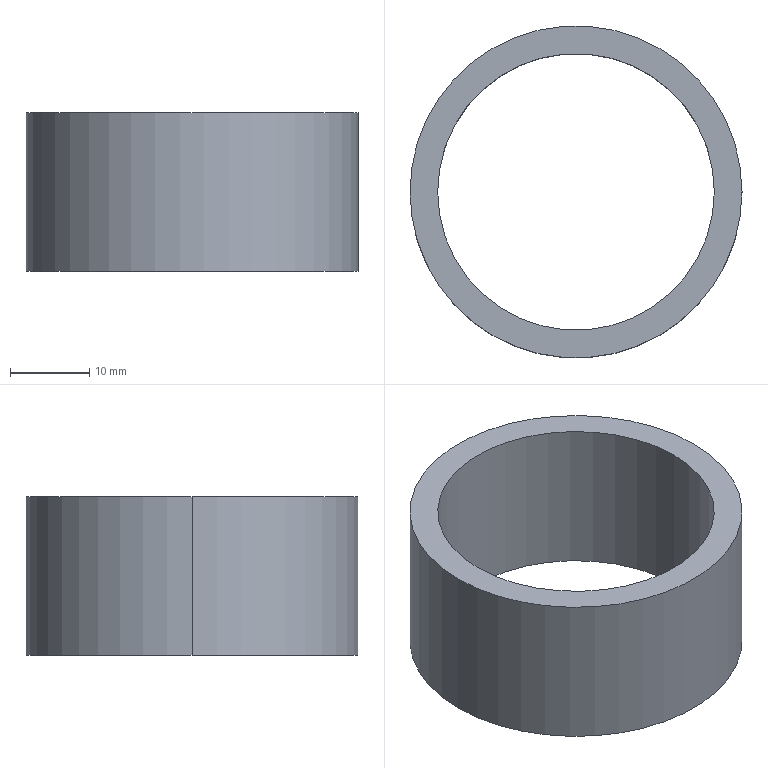Part | SolidWorks | features BaseBody 1 | 1 solid | 6 faces | box 42 x 42 x 20 mm | volume 8467 mm3 | cylinder 4 | plane 2 | commonest cylinder face diameters 35 x2 42 x2
STEP:
#1=CARTESIAN_POINT('',(323.083,269.388,51.922));
#2=VERTEX_POINT('',#1);
#3=CARTESIAN_POINT('',(358.083,269.388,51.922));
#4=VERTEX_POINT('',#3);
#5=CARTESIAN_POINT('',(340.583,269.388,51.922));
#6=DIRECTION('',(0.,0.,1.));
#7=DIRECTION('',(0.,-1.,0.));
#8=AXIS2_PLACEMENT_3D('',#5,#6,#7);
#9=CIRCLE('',#8,17.5);
#10=EDGE_CURVE('',#2,#4,#9,.T.);
#11=ORIENTED_EDGE('',*,*,#10,.F.);
#12=CARTESIAN_POINT('',(323.083,269.388,71.922));
#13=VERTEX_POINT('',#12);
#14=CARTESIAN_POINT('',(323.083,269.388,52.471));
#15=DIRECTION('',(0.,0.,1.));
#16=VECTOR('',#15,1000.);
#17=LINE('',#14,#16);
#18=EDGE_CURVE('',#2,#13,#17,.T.);
#19=ORIENTED_EDGE('',*,*,#18,.T.);
#20=CARTESIAN_POINT('',(358.083,269.388,71.922));
#21=VERTEX_POINT('',#20);
#22=CARTESIAN_POINT('',(340.583,269.388,71.922));
#23=DIRECTION('',(0.,0.,-1.));
#24=DIRECTION('',(-1.,0.,0.));
#25=AXIS2_PLACEMENT_3D('',#22,#23,#24);
#26=CIRCLE('',#25,17.5);
#27=EDGE_CURVE('',#21,#13,#26,.T.);
#28=ORIENTED_EDGE('',*,*,#27,.F.);
#29=CARTESIAN_POINT('',(358.083,269.388,52.471));
#30=DIRECTION('',(0.,0.,1.));
#31=VECTOR('',#30,1000.);
#32=LINE('',#29,#31);
#33=EDGE_CURVE('',#4,#21,#32,.T.);
#34=ORIENTED_EDGE('',*,*,#33,.F.);
#35=EDGE_LOOP('',(#11,#19,#28,#34));
#36=FACE_OUTER_BOUND('',#35,.T.);
#37=CARTESIAN_POINT('',(340.583,269.388,52.471));
#38=DIRECTION('',(0.,0.,1.));
#39=DIRECTION('',(1.,0.,0.));
#40=AXIS2_PLACEMENT_3D('',#37,#38,#39);
#41=CYLINDRICAL_SURFACE('',#40,17.5);
#42=ADVANCED_FACE('',(#36),#41,.F.);
#43=CARTESIAN_POINT('',(319.583,269.388,51.922));
#44=VERTEX_POINT('',#43);
#45=CARTESIAN_POINT('',(361.583,269.388,51.922));
#46=VERTEX_POINT('',#45);
#47=CARTESIAN_POINT('',(340.583,269.388,51.922));
#48=DIRECTION('',(0.,0.,-1.));
#49=DIRECTION('',(1.,0.,0.));
#50=AXIS2_PLACEMENT_3D('',#47,#48,#49);
#51=CIRCLE('',#50,21.);
#52=EDGE_CURVE('',#44,#46,#51,.T.);
#53=ORIENTED_EDGE('',*,*,#52,.F.);
#54=CARTESIAN_POINT('',(319.583,269.388,71.922));
#55=VERTEX_POINT('',#54);
#56=CARTESIAN_POINT('',(319.583,269.388,52.471));
#57=DIRECTION('',(0.,0.,1.));
#58=VECTOR('',#57,1000.);
#59=LINE('',#56,#58);
#60=EDGE_CURVE('',#44,#55,#59,.T.);
#61=ORIENTED_EDGE('',*,*,#60,.T.);
#62=CARTESIAN_POINT('',(361.583,269.388,71.922));
#63=VERTEX_POINT('',#62);
#64=CARTESIAN_POINT('',(340.583,269.388,71.922));
#65=DIRECTION('',(0.,0.,1.));
#66=DIRECTION('',(1.,0.,0.));
#67=AXIS2_PLACEMENT_3D('',#64,#65,#66);
#68=CIRCLE('',#67,21.);
#69=EDGE_CURVE('',#63,#55,#68,.T.);
#70=ORIENTED_EDGE('',*,*,#69,.F.);
#71=CARTESIAN_POINT('',(361.583,269.388,52.471));
#72=DIRECTION('',(0.,0.,1.));
#73=VECTOR('',#72,1000.);
#74=LINE('',#71,#73);
#75=EDGE_CURVE('',#46,#63,#74,.T.);
#76=ORIENTED_EDGE('',*,*,#75,.F.);
#77=EDGE_LOOP('',(#53,#61,#70,#76));
#78=FACE_OUTER_BOUND('',#77,.T.);
#79=CARTESIAN_POINT('',(340.583,269.388,52.471));
#80=DIRECTION('',(0.,0.,1.));
#81=DIRECTION('',(1.,0.,0.));
#82=AXIS2_PLACEMENT_3D('',#79,#80,#81);
#83=CYLINDRICAL_SURFACE('',#82,21.);
#84=ADVANCED_FACE('',(#78),#83,.T.);
#85=ORIENTED_EDGE('',*,*,#60,.F.);
#86=CARTESIAN_POINT('',(340.583,269.388,51.922));
#87=DIRECTION('',(0.,0.,-1.));
#88=DIRECTION('',(1.,0.,0.));
#89=AXIS2_PLACEMENT_3D('',#86,#87,#88);
#90=CIRCLE('',#89,21.);
#91=EDGE_CURVE('',#46,#44,#90,.T.);
#92=ORIENTED_EDGE('',*,*,#91,.F.);
#93=ORIENTED_EDGE('',*,*,#75,.T.);
#94=CARTESIAN_POINT('',(340.583,269.388,71.922));
#95=DIRECTION('',(0.,0.,1.));
#96=DIRECTION('',(1.,0.,0.));
#97=AXIS2_PLACEMENT_3D('',#94,#95,#96);
#98=CIRCLE('',#97,21.);
#99=EDGE_CURVE('',#55,#63,#98,.T.);
#100=ORIENTED_EDGE('',*,*,#99,.F.);
#101=EDGE_LOOP('',(#85,#92,#93,#100));
#102=FACE_OUTER_BOUND('',#101,.T.);
#103=CARTESIAN_POINT('',(340.583,269.388,52.471));
#104=DIRECTION('',(0.,0.,1.));
#105=DIRECTION('',(1.,0.,0.));
#106=AXIS2_PLACEMENT_3D('',#103,#104,#105);
#107=CYLINDRICAL_SURFACE('',#106,21.);
#108=ADVANCED_FACE('',(#102),#107,.T.);
#109=CARTESIAN_POINT('',(340.583,269.388,51.922));
#110=DIRECTION('',(0.,0.,1.));
#111=DIRECTION('',(0.,-1.,0.));
#112=AXIS2_PLACEMENT_3D('',#109,#110,#111);
#113=CIRCLE('',#112,17.5);
#114=EDGE_CURVE('',#4,#2,#113,.T.);
#115=ORIENTED_EDGE('',*,*,#114,.T.);
#116=ORIENTED_EDGE('',*,*,#10,.T.);
#117=EDGE_LOOP('',(#115,#116));
#118=FACE_BOUND('',#117,.T.);
#119=ORIENTED_EDGE('',*,*,#91,.T.);
#120=ORIENTED_EDGE('',*,*,#52,.T.);
#121=EDGE_LOOP('',(#119,#120));
#122=FACE_OUTER_BOUND('',#121,.T.);
#123=CARTESIAN_POINT('',(340.583,269.388,51.922));
#124=DIRECTION('',(0.,0.,-1.));
#125=DIRECTION('',(-1.,0.,0.));
#126=AXIS2_PLACEMENT_3D('',#123,#124,#125);
#127=PLANE('',#126);
#128=ADVANCED_FACE('',(#118,#122),#127,.T.);
#129=ORIENTED_EDGE('',*,*,#18,.F.);
#130=ORIENTED_EDGE('',*,*,#114,.F.);
#131=ORIENTED_EDGE('',*,*,#33,.T.);
#132=CARTESIAN_POINT('',(340.583,269.388,71.922));
#133=DIRECTION('',(0.,0.,-1.));
#134=DIRECTION('',(-1.,0.,0.));
#135=AXIS2_PLACEMENT_3D('',#132,#133,#134);
#136=CIRCLE('',#135,17.5);
#137=EDGE_CURVE('',#13,#21,#136,.T.);
#138=ORIENTED_EDGE('',*,*,#137,.F.);
#139=EDGE_LOOP('',(#129,#130,#131,#138));
#140=FACE_OUTER_BOUND('',#139,.T.);
#141=CARTESIAN_POINT('',(340.583,269.388,52.471));
#142=DIRECTION('',(0.,0.,1.));
#143=DIRECTION('',(1.,0.,0.));
#144=AXIS2_PLACEMENT_3D('',#141,#142,#143);
#145=CYLINDRICAL_SURFACE('',#144,17.5);
#146=ADVANCED_FACE('',(#140),#145,.F.);
#147=ORIENTED_EDGE('',*,*,#27,.T.);
#148=ORIENTED_EDGE('',*,*,#137,.T.);
#149=EDGE_LOOP('',(#147,#148));
#150=FACE_BOUND('',#149,.T.);
#151=ORIENTED_EDGE('',*,*,#69,.T.);
#152=ORIENTED_EDGE('',*,*,#99,.T.);
#153=EDGE_LOOP('',(#151,#152));
#154=FACE_OUTER_BOUND('',#153,.T.);
#155=CARTESIAN_POINT('',(340.583,269.388,71.922));
#156=DIRECTION('',(0.,0.,1.));
#157=DIRECTION('',(0.,-1.,0.));
#158=AXIS2_PLACEMENT_3D('',#155,#156,#157);
#159=PLANE('',#158);
#160=ADVANCED_FACE('',(#150,#154),#159,.T.);
#161=CLOSED_SHELL('',(#42,#84,#108,#128,#146,#160));
#162=MANIFOLD_SOLID_BREP('',#161);
#163=CARTESIAN_POINT('',(0.,0.,0.));
#164=DIRECTION('',(0.,0.,1.));
#165=DIRECTION('',(1.,0.,0.));
#166=AXIS2_PLACEMENT_3D('',#163,#164,#165);
#167=(LENGTH_UNIT()NAMED_UNIT(*)SI_UNIT(.MILLI.,.METRE.));
#168=UNCERTAINTY_MEASURE_WITH_UNIT(LENGTH_MEASURE(0.00001),#167,'','');
#169=(NAMED_UNIT(*)PLANE_ANGLE_UNIT()SI_UNIT($,.RADIAN.));
#170=(NAMED_UNIT(*)SI_UNIT($,.STERADIAN.)SOLID_ANGLE_UNIT());
#171=(GEOMETRIC_REPRESENTATION_CONTEXT(3)GLOBAL_UNCERTAINTY_ASSIGNED_CONTEXT((#168))GLOBAL_UNIT_ASSIGNED_CONTEXT((#167,#169,#170))REPRESENTATION_CONTEXT('',''));
#172=ADVANCED_BREP_SHAPE_REPRESENTATION('',(#162,#166),#171);